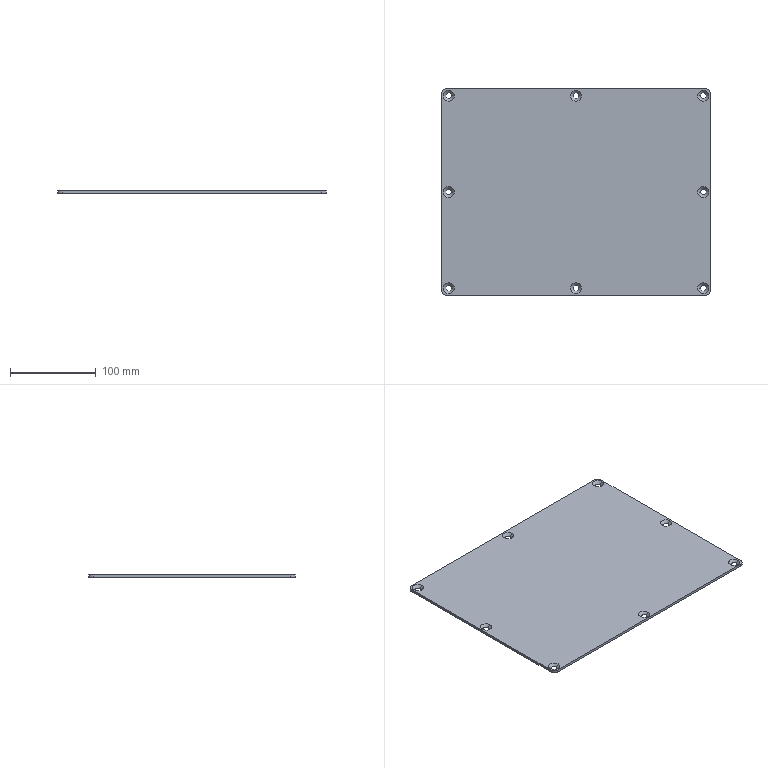Part | STEP file | PN_0001-11 Cover plate A | 1 solid | 26 faces | box 312 x 240 x 3 mm | volume 222709 mm3 | cone 16 | plane 6 | cylinder 4 | commonest cylinder face diameters 10 x4
STEP:
#1=CARTESIAN_POINT('',(-151.4,112.,0.));
#2=VERTEX_POINT('',#1);
#3=CARTESIAN_POINT('',(-144.6,112.,0.));
#4=VERTEX_POINT('',#3);
#5=CARTESIAN_POINT('',(-148.,112.,0.));
#6=DIRECTION('',(0.,0.,1.));
#7=DIRECTION('',(1.,0.,0.));
#8=AXIS2_PLACEMENT_3D('',#5,#6,#7);
#9=CIRCLE('',#8,3.4);
#10=EDGE_CURVE('',#2,#4,#9,.T.);
#11=ORIENTED_EDGE('',*,*,#10,.F.);
#12=CARTESIAN_POINT('',(-154.4,112.,3.));
#13=VERTEX_POINT('',#12);
#14=CARTESIAN_POINT('',(-154.4,112.,3.));
#15=DIRECTION('',(-0.7071,0.,0.7071));
#16=VECTOR('',#15,1000.);
#17=LINE('',#14,#16);
#18=EDGE_CURVE('',#2,#13,#17,.T.);
#19=ORIENTED_EDGE('',*,*,#18,.T.);
#20=CARTESIAN_POINT('',(-141.6,112.,3.));
#21=VERTEX_POINT('',#20);
#22=CARTESIAN_POINT('',(-148.,112.,3.));
#23=DIRECTION('',(0.,0.,1.));
#24=DIRECTION('',(1.,0.,0.));
#25=AXIS2_PLACEMENT_3D('',#22,#23,#24);
#26=CIRCLE('',#25,6.4);
#27=EDGE_CURVE('',#13,#21,#26,.T.);
#28=ORIENTED_EDGE('',*,*,#27,.T.);
#29=CARTESIAN_POINT('',(-141.6,112.,3.));
#30=DIRECTION('',(0.7071,0.,0.7071));
#31=VECTOR('',#30,1000.);
#32=LINE('',#29,#31);
#33=EDGE_CURVE('',#4,#21,#32,.T.);
#34=ORIENTED_EDGE('',*,*,#33,.F.);
#35=EDGE_LOOP('',(#11,#19,#28,#34));
#36=FACE_OUTER_BOUND('',#35,.T.);
#37=CARTESIAN_POINT('',(-148.,112.,3.));
#38=DIRECTION('',(0.,0.,1.));
#39=DIRECTION('',(1.,0.,0.));
#40=AXIS2_PLACEMENT_3D('',#37,#38,#39);
#41=CONICAL_SURFACE('',#40,6.4,0.7854);
#42=ADVANCED_FACE('',(#36),#41,.F.);
#43=CARTESIAN_POINT('',(-3.4,112.,0.));
#44=VERTEX_POINT('',#43);
#45=CARTESIAN_POINT('',(3.4,112.,0.));
#46=VERTEX_POINT('',#45);
#47=CARTESIAN_POINT('',(0.,112.,0.));
#48=DIRECTION('',(0.,0.,1.));
#49=DIRECTION('',(1.,0.,0.));
#50=AXIS2_PLACEMENT_3D('',#47,#48,#49);
#51=CIRCLE('',#50,3.4);
#52=EDGE_CURVE('',#44,#46,#51,.T.);
#53=ORIENTED_EDGE('',*,*,#52,.F.);
#54=CARTESIAN_POINT('',(-6.4,112.,3.));
#55=VERTEX_POINT('',#54);
#56=CARTESIAN_POINT('',(-6.4,112.,3.));
#57=DIRECTION('',(-0.7071,0.,0.7071));
#58=VECTOR('',#57,1000.);
#59=LINE('',#56,#58);
#60=EDGE_CURVE('',#44,#55,#59,.T.);
#61=ORIENTED_EDGE('',*,*,#60,.T.);
#62=CARTESIAN_POINT('',(6.4,112.,3.));
#63=VERTEX_POINT('',#62);
#64=CARTESIAN_POINT('',(0.,112.,3.));
#65=DIRECTION('',(0.,0.,1.));
#66=DIRECTION('',(1.,0.,0.));
#67=AXIS2_PLACEMENT_3D('',#64,#65,#66);
#68=CIRCLE('',#67,6.4);
#69=EDGE_CURVE('',#55,#63,#68,.T.);
#70=ORIENTED_EDGE('',*,*,#69,.T.);
#71=CARTESIAN_POINT('',(6.4,112.,3.));
#72=DIRECTION('',(0.7071,0.,0.7071));
#73=VECTOR('',#72,1000.);
#74=LINE('',#71,#73);
#75=EDGE_CURVE('',#46,#63,#74,.T.);
#76=ORIENTED_EDGE('',*,*,#75,.F.);
#77=EDGE_LOOP('',(#53,#61,#70,#76));
#78=FACE_OUTER_BOUND('',#77,.T.);
#79=CARTESIAN_POINT('',(0.,112.,3.));
#80=DIRECTION('',(0.,0.,1.));
#81=DIRECTION('',(1.,0.,0.));
#82=AXIS2_PLACEMENT_3D('',#79,#80,#81);
#83=CONICAL_SURFACE('',#82,6.4,0.7854);
#84=ADVANCED_FACE('',(#78),#83,.F.);
#85=CARTESIAN_POINT('',(144.6,112.,0.));
#86=VERTEX_POINT('',#85);
#87=CARTESIAN_POINT('',(151.4,112.,0.));
#88=VERTEX_POINT('',#87);
#89=CARTESIAN_POINT('',(148.,112.,0.));
#90=DIRECTION('',(0.,0.,1.));
#91=DIRECTION('',(1.,0.,0.));
#92=AXIS2_PLACEMENT_3D('',#89,#90,#91);
#93=CIRCLE('',#92,3.4);
#94=EDGE_CURVE('',#86,#88,#93,.T.);
#95=ORIENTED_EDGE('',*,*,#94,.F.);
#96=CARTESIAN_POINT('',(141.6,112.,3.));
#97=VERTEX_POINT('',#96);
#98=CARTESIAN_POINT('',(141.6,112.,3.));
#99=DIRECTION('',(-0.7071,0.,0.7071));
#100=VECTOR('',#99,1000.);
#101=LINE('',#98,#100);
#102=EDGE_CURVE('',#86,#97,#101,.T.);
#103=ORIENTED_EDGE('',*,*,#102,.T.);
#104=CARTESIAN_POINT('',(154.4,112.,3.));
#105=VERTEX_POINT('',#104);
#106=CARTESIAN_POINT('',(148.,112.,3.));
#107=DIRECTION('',(0.,0.,1.));
#108=DIRECTION('',(1.,0.,0.));
#109=AXIS2_PLACEMENT_3D('',#106,#107,#108);
#110=CIRCLE('',#109,6.4);
#111=EDGE_CURVE('',#97,#105,#110,.T.);
#112=ORIENTED_EDGE('',*,*,#111,.T.);
#113=CARTESIAN_POINT('',(154.4,112.,3.));
#114=DIRECTION('',(0.7071,0.,0.7071));
#115=VECTOR('',#114,1000.);
#116=LINE('',#113,#115);
#117=EDGE_CURVE('',#88,#105,#116,.T.);
#118=ORIENTED_EDGE('',*,*,#117,.F.);
#119=EDGE_LOOP('',(#95,#103,#112,#118));
#120=FACE_OUTER_BOUND('',#119,.T.);
#121=CARTESIAN_POINT('',(148.,112.,3.));
#122=DIRECTION('',(0.,0.,1.));
#123=DIRECTION('',(1.,0.,0.));
#124=AXIS2_PLACEMENT_3D('',#121,#122,#123);
#125=CONICAL_SURFACE('',#124,6.4,0.7854);
#126=ADVANCED_FACE('',(#120),#125,.F.);
#127=CARTESIAN_POINT('',(144.6,0.,0.));
#128=VERTEX_POINT('',#127);
#129=CARTESIAN_POINT('',(151.4,0.,0.));
#130=VERTEX_POINT('',#129);
#131=CARTESIAN_POINT('',(148.,0.,0.));
#132=DIRECTION('',(0.,0.,1.));
#133=DIRECTION('',(1.,0.,0.));
#134=AXIS2_PLACEMENT_3D('',#131,#132,#133);
#135=CIRCLE('',#134,3.4);
#136=EDGE_CURVE('',#128,#130,#135,.T.);
#137=ORIENTED_EDGE('',*,*,#136,.F.);
#138=CARTESIAN_POINT('',(141.6,0.,3.));
#139=VERTEX_POINT('',#138);
#140=CARTESIAN_POINT('',(141.6,0.,3.));
#141=DIRECTION('',(-0.7071,0.,0.7071));
#142=VECTOR('',#141,1000.);
#143=LINE('',#140,#142);
#144=EDGE_CURVE('',#128,#139,#143,.T.);
#145=ORIENTED_EDGE('',*,*,#144,.T.);
#146=CARTESIAN_POINT('',(154.4,0.,3.));
#147=VERTEX_POINT('',#146);
#148=CARTESIAN_POINT('',(148.,0.,3.));
#149=DIRECTION('',(0.,0.,1.));
#150=DIRECTION('',(1.,0.,0.));
#151=AXIS2_PLACEMENT_3D('',#148,#149,#150);
#152=CIRCLE('',#151,6.4);
#153=EDGE_CURVE('',#139,#147,#152,.T.);
#154=ORIENTED_EDGE('',*,*,#153,.T.);
#155=CARTESIAN_POINT('',(154.4,0.,3.));
#156=DIRECTION('',(0.7071,0.,0.7071));
#157=VECTOR('',#156,1000.);
#158=LINE('',#155,#157);
#159=EDGE_CURVE('',#130,#147,#158,.T.);
#160=ORIENTED_EDGE('',*,*,#159,.F.);
#161=EDGE_LOOP('',(#137,#145,#154,#160));
#162=FACE_OUTER_BOUND('',#161,.T.);
#163=CARTESIAN_POINT('',(148.,0.,3.));
#164=DIRECTION('',(0.,0.,1.));
#165=DIRECTION('',(1.,0.,0.));
#166=AXIS2_PLACEMENT_3D('',#163,#164,#165);
#167=CONICAL_SURFACE('',#166,6.4,0.7854);
#168=ADVANCED_FACE('',(#162),#167,.F.);
#169=CARTESIAN_POINT('',(144.6,-112.,0.));
#170=VERTEX_POINT('',#169);
#171=CARTESIAN_POINT('',(151.4,-112.,0.));
#172=VERTEX_POINT('',#171);
#173=CARTESIAN_POINT('',(148.,-112.,0.));
#174=DIRECTION('',(0.,0.,1.));
#175=DIRECTION('',(1.,0.,0.));
#176=AXIS2_PLACEMENT_3D('',#173,#174,#175);
#177=CIRCLE('',#176,3.4);
#178=EDGE_CURVE('',#170,#172,#177,.T.);
#179=ORIENTED_EDGE('',*,*,#178,.F.);
#180=CARTESIAN_POINT('',(141.6,-112.,3.));
#181=VERTEX_POINT('',#180);
#182=CARTESIAN_POINT('',(141.6,-112.,3.));
#183=DIRECTION('',(-0.7071,0.,0.7071));
#184=VECTOR('',#183,1000.);
#185=LINE('',#182,#184);
#186=EDGE_CURVE('',#170,#181,#185,.T.);
#187=ORIENTED_EDGE('',*,*,#186,.T.);
#188=CARTESIAN_POINT('',(154.4,-112.,3.));
#189=VERTEX_POINT('',#188);
#190=CARTESIAN_POINT('',(148.,-112.,3.));
#191=DIRECTION('',(0.,0.,1.));
#192=DIRECTION('',(1.,0.,0.));
#193=AXIS2_PLACEMENT_3D('',#190,#191,#192);
#194=CIRCLE('',#193,6.4);
#195=EDGE_CURVE('',#181,#189,#194,.T.);
#196=ORIENTED_EDGE('',*,*,#195,.T.);
#197=CARTESIAN_POINT('',(154.4,-112.,3.));
#198=DIRECTION('',(0.7071,0.,0.7071));
#199=VECTOR('',#198,1000.);
#200=LINE('',#197,#199);
#201=EDGE_CURVE('',#172,#189,#200,.T.);
#202=ORIENTED_EDGE('',*,*,#201,.F.);
#203=EDGE_LOOP('',(#179,#187,#196,#202));
#204=FACE_OUTER_BOUND('',#203,.T.);
#205=CARTESIAN_POINT('',(148.,-112.,3.));
#206=DIRECTION('',(0.,0.,1.));
#207=DIRECTION('',(1.,0.,0.));
#208=AXIS2_PLACEMENT_3D('',#205,#206,#207);
#209=CONICAL_SURFACE('',#208,6.4,0.7854);
#210=ADVANCED_FACE('',(#204),#209,.F.);
#211=CARTESIAN_POINT('',(-3.4,-112.,0.));
#212=VERTEX_POINT('',#211);
#213=CARTESIAN_POINT('',(3.4,-112.,0.));
#214=VERTEX_POINT('',#213);
#215=CARTESIAN_POINT('',(0.,-112.,0.));
#216=DIRECTION('',(0.,0.,1.));
#217=DIRECTION('',(1.,0.,0.));
#218=AXIS2_PLACEMENT_3D('',#215,#216,#217);
#219=CIRCLE('',#218,3.4);
#220=EDGE_CURVE('',#212,#214,#219,.T.);
#221=ORIENTED_EDGE('',*,*,#220,.F.);
#222=CARTESIAN_POINT('',(-6.4,-112.,3.));
#223=VERTEX_POINT('',#222);
#224=CARTESIAN_POINT('',(-6.4,-112.,3.));
#225=DIRECTION('',(-0.7071,0.,0.7071));
#226=VECTOR('',#225,1000.);
#227=LINE('',#224,#226);
#228=EDGE_CURVE('',#212,#223,#227,.T.);
#229=ORIENTED_EDGE('',*,*,#228,.T.);
#230=CARTESIAN_POINT('',(6.4,-112.,3.));
#231=VERTEX_POINT('',#230);
#232=CARTESIAN_POINT('',(0.,-112.,3.));
#233=DIRECTION('',(0.,0.,1.));
#234=DIRECTION('',(1.,0.,0.));
#235=AXIS2_PLACEMENT_3D('',#232,#233,#234);
#236=CIRCLE('',#235,6.4);
#237=EDGE_CURVE('',#223,#231,#236,.T.);
#238=ORIENTED_EDGE('',*,*,#237,.T.);
#239=CARTESIAN_POINT('',(6.4,-112.,3.));
#240=DIRECTION('',(0.7071,0.,0.7071));
#241=VECTOR('',#240,1000.);
#242=LINE('',#239,#241);
#243=EDGE_CURVE('',#214,#231,#242,.T.);
#244=ORIENTED_EDGE('',*,*,#243,.F.);
#245=EDGE_LOOP('',(#221,#229,#238,#244));
#246=FACE_OUTER_BOUND('',#245,.T.);
#247=CARTESIAN_POINT('',(0.,-112.,3.));
#248=DIRECTION('',(0.,0.,1.));
#249=DIRECTION('',(1.,0.,0.));
#250=AXIS2_PLACEMENT_3D('',#247,#248,#249);
#251=CONICAL_SURFACE('',#250,6.4,0.7854);
#252=ADVANCED_FACE('',(#246),#251,.F.);
#253=CARTESIAN_POINT('',(-151.4,-112.,0.));
#254=VERTEX_POINT('',#253);
#255=CARTESIAN_POINT('',(-144.6,-112.,0.));
#256=VERTEX_POINT('',#255);
#257=CARTESIAN_POINT('',(-148.,-112.,0.));
#258=DIRECTION('',(0.,0.,1.));
#259=DIRECTION('',(1.,0.,0.));
#260=AXIS2_PLACEMENT_3D('',#257,#258,#259);
#261=CIRCLE('',#260,3.4);
#262=EDGE_CURVE('',#254,#256,#261,.T.);
#263=ORIENTED_EDGE('',*,*,#262,.F.);
#264=CARTESIAN_POINT('',(-154.4,-112.,3.));
#265=VERTEX_POINT('',#264);
#266=CARTESIAN_POINT('',(-154.4,-112.,3.));
#267=DIRECTION('',(-0.7071,0.,0.7071));
#268=VECTOR('',#267,1000.);
#269=LINE('',#266,#268);
#270=EDGE_CURVE('',#254,#265,#269,.T.);
#271=ORIENTED_EDGE('',*,*,#270,.T.);
#272=CARTESIAN_POINT('',(-141.6,-112.,3.));
#273=VERTEX_POINT('',#272);
#274=CARTESIAN_POINT('',(-148.,-112.,3.));
#275=DIRECTION('',(0.,0.,1.));
#276=DIRECTION('',(1.,0.,0.));
#277=AXIS2_PLACEMENT_3D('',#274,#275,#276);
#278=CIRCLE('',#277,6.4);
#279=EDGE_CURVE('',#265,#273,#278,.T.);
#280=ORIENTED_EDGE('',*,*,#279,.T.);
#281=CARTESIAN_POINT('',(-141.6,-112.,3.));
#282=DIRECTION('',(0.7071,0.,0.7071));
#283=VECTOR('',#282,1000.);
#284=LINE('',#281,#283);
#285=EDGE_CURVE('',#256,#273,#284,.T.);
#286=ORIENTED_EDGE('',*,*,#285,.F.);
#287=EDGE_LOOP('',(#263,#271,#280,#286));
#288=FACE_OUTER_BOUND('',#287,.T.);
#289=CARTESIAN_POINT('',(-148.,-112.,3.));
#290=DIRECTION('',(0.,0.,1.));
#291=DIRECTION('',(1.,0.,0.));
#292=AXIS2_PLACEMENT_3D('',#289,#290,#291);
#293=CONICAL_SURFACE('',#292,6.4,0.7854);
#294=ADVANCED_FACE('',(#288),#293,.F.);
#295=CARTESIAN_POINT('',(-151.4,0.,0.));
#296=VERTEX_POINT('',#295);
#297=CARTESIAN_POINT('',(-144.6,0.,0.));
#298=VERTEX_POINT('',#297);
#299=CARTESIAN_POINT('',(-148.,0.,0.));
#300=DIRECTION('',(0.,0.,1.));
#301=DIRECTION('',(1.,0.,0.));
#302=AXIS2_PLACEMENT_3D('',#299,#300,#301);
#303=CIRCLE('',#302,3.4);
#304=EDGE_CURVE('',#296,#298,#303,.T.);
#305=ORIENTED_EDGE('',*,*,#304,.F.);
#306=CARTESIAN_POINT('',(-154.4,0.,3.));
#307=VERTEX_POINT('',#306);
#308=CARTESIAN_POINT('',(-154.4,0.,3.));
#309=DIRECTION('',(-0.7071,0.,0.7071));
#310=VECTOR('',#309,1000.);
#311=LINE('',#308,#310);
#312=EDGE_CURVE('',#296,#307,#311,.T.);
#313=ORIENTED_EDGE('',*,*,#312,.T.);
#314=CARTESIAN_POINT('',(-141.6,0.,3.));
#315=VERTEX_POINT('',#314);
#316=CARTESIAN_POINT('',(-148.,0.,3.));
#317=DIRECTION('',(0.,0.,1.));
#318=DIRECTION('',(1.,0.,0.));
#319=AXIS2_PLACEMENT_3D('',#316,#317,#318);
#320=CIRCLE('',#319,6.4);
#321=EDGE_CURVE('',#307,#315,#320,.T.);
#322=ORIENTED_EDGE('',*,*,#321,.T.);
#323=CARTESIAN_POINT('',(-141.6,0.,3.));
#324=DIRECTION('',(0.7071,0.,0.7071));
#325=VECTOR('',#324,1000.);
#326=LINE('',#323,#325);
#327=EDGE_CURVE('',#298,#315,#326,.T.);
#328=ORIENTED_EDGE('',*,*,#327,.F.);
#329=EDGE_LOOP('',(#305,#313,#322,#328));
#330=FACE_OUTER_BOUND('',#329,.T.);
#331=CARTESIAN_POINT('',(-148.,0.,3.));
#332=DIRECTION('',(0.,0.,1.));
#333=DIRECTION('',(1.,0.,0.));
#334=AXIS2_PLACEMENT_3D('',#331,#332,#333);
#335=CONICAL_SURFACE('',#334,6.4,0.7854);
#336=ADVANCED_FACE('',(#330),#335,.F.);
#337=CARTESIAN_POINT('',(-156.,115.,0.));
#338=VERTEX_POINT('',#337);
#339=CARTESIAN_POINT('',(-156.,-115.,0.));
#340=VERTEX_POINT('',#339);
#341=CARTESIAN_POINT('',(-156.,-120.,0.));
#342=DIRECTION('',(0.,-1.,0.));
#343=VECTOR('',#342,1000.);
#344=LINE('',#341,#343);
#345=EDGE_CURVE('',#338,#340,#344,.T.);
#346=ORIENTED_EDGE('',*,*,#345,.T.);
#347=CARTESIAN_POINT('',(-156.,-115.,3.));
#348=VERTEX_POINT('',#347);
#349=CARTESIAN_POINT('',(-156.,-115.,3.));
#350=DIRECTION('',(0.,0.,1.));
#351=VECTOR('',#350,1000.);
#352=LINE('',#349,#351);
#353=EDGE_CURVE('',#340,#348,#352,.T.);
#354=ORIENTED_EDGE('',*,*,#353,.T.);
#355=CARTESIAN_POINT('',(-156.,115.,3.));
#356=VERTEX_POINT('',#355);
#357=CARTESIAN_POINT('',(-156.,-120.,3.));
#358=DIRECTION('',(0.,-1.,0.));
#359=VECTOR('',#358,1000.);
#360=LINE('',#357,#359);
#361=EDGE_CURVE('',#356,#348,#360,.T.);
#362=ORIENTED_EDGE('',*,*,#361,.F.);
#363=CARTESIAN_POINT('',(-156.,115.,3.));
#364=DIRECTION('',(0.,0.,-1.));
#365=VECTOR('',#364,1000.);
#366=LINE('',#363,#365);
#367=EDGE_CURVE('',#356,#338,#366,.T.);
#368=ORIENTED_EDGE('',*,*,#367,.T.);
#369=EDGE_LOOP('',(#346,#354,#362,#368));
#370=FACE_OUTER_BOUND('',#369,.T.);
#371=CARTESIAN_POINT('',(-156.,-120.,3.));
#372=DIRECTION('',(1.,0.,0.));
#373=DIRECTION('',(0.,0.,-1.));
#374=AXIS2_PLACEMENT_3D('',#371,#372,#373);
#375=PLANE('',#374);
#376=ADVANCED_FACE('',(#370),#375,.F.);
#377=CARTESIAN_POINT('',(-151.,-120.,0.));
#378=VERTEX_POINT('',#377);
#379=CARTESIAN_POINT('',(151.,-120.,0.));
#380=VERTEX_POINT('',#379);
#381=CARTESIAN_POINT('',(156.,-120.,0.));
#382=DIRECTION('',(1.,0.,0.));
#383=VECTOR('',#382,1000.);
#384=LINE('',#381,#383);
#385=EDGE_CURVE('',#378,#380,#384,.T.);
#386=ORIENTED_EDGE('',*,*,#385,.T.);
#387=CARTESIAN_POINT('',(151.,-120.,3.));
#388=VERTEX_POINT('',#387);
#389=CARTESIAN_POINT('',(151.,-120.,3.));
#390=DIRECTION('',(0.,0.,1.));
#391=VECTOR('',#390,1000.);
#392=LINE('',#389,#391);
#393=EDGE_CURVE('',#380,#388,#392,.T.);
#394=ORIENTED_EDGE('',*,*,#393,.T.);
#395=CARTESIAN_POINT('',(-151.,-120.,3.));
#396=VERTEX_POINT('',#395);
#397=CARTESIAN_POINT('',(156.,-120.,3.));
#398=DIRECTION('',(1.,0.,0.));
#399=VECTOR('',#398,1000.);
#400=LINE('',#397,#399);
#401=EDGE_CURVE('',#396,#388,#400,.T.);
#402=ORIENTED_EDGE('',*,*,#401,.F.);
#403=CARTESIAN_POINT('',(-151.,-120.,3.));
#404=DIRECTION('',(0.,0.,-1.));
#405=VECTOR('',#404,1000.);
#406=LINE('',#403,#405);
#407=EDGE_CURVE('',#396,#378,#406,.T.);
#408=ORIENTED_EDGE('',*,*,#407,.T.);
#409=EDGE_LOOP('',(#386,#394,#402,#408));
#410=FACE_OUTER_BOUND('',#409,.T.);
#411=CARTESIAN_POINT('',(156.,-120.,3.));
#412=DIRECTION('',(0.,1.,0.));
#413=DIRECTION('',(0.,0.,1.));
#414=AXIS2_PLACEMENT_3D('',#411,#412,#413);
#415=PLANE('',#414);
#416=ADVANCED_FACE('',(#410),#415,.F.);
#417=CARTESIAN_POINT('',(156.,-115.,3.));
#418=VERTEX_POINT('',#417);
#419=CARTESIAN_POINT('',(156.,115.,3.));
#420=VERTEX_POINT('',#419);
#421=CARTESIAN_POINT('',(156.,-120.,3.));
#422=DIRECTION('',(0.,1.,0.));
#423=VECTOR('',#422,1000.);
#424=LINE('',#421,#423);
#425=EDGE_CURVE('',#418,#420,#424,.T.);
#426=ORIENTED_EDGE('',*,*,#425,.F.);
#427=CARTESIAN_POINT('',(156.,-115.,0.));
#428=VERTEX_POINT('',#427);
#429=CARTESIAN_POINT('',(156.,-115.,3.));
#430=DIRECTION('',(0.,0.,-1.));
#431=VECTOR('',#430,1000.);
#432=LINE('',#429,#431);
#433=EDGE_CURVE('',#418,#428,#432,.T.);
#434=ORIENTED_EDGE('',*,*,#433,.T.);
#435=CARTESIAN_POINT('',(156.,115.,0.));
#436=VERTEX_POINT('',#435);
#437=CARTESIAN_POINT('',(156.,-120.,0.));
#438=DIRECTION('',(0.,1.,0.));
#439=VECTOR('',#438,1000.);
#440=LINE('',#437,#439);
#441=EDGE_CURVE('',#428,#436,#440,.T.);
#442=ORIENTED_EDGE('',*,*,#441,.T.);
#443=CARTESIAN_POINT('',(156.,115.,3.));
#444=DIRECTION('',(0.,0.,1.));
#445=VECTOR('',#444,1000.);
#446=LINE('',#443,#445);
#447=EDGE_CURVE('',#436,#420,#446,.T.);
#448=ORIENTED_EDGE('',*,*,#447,.T.);
#449=EDGE_LOOP('',(#426,#434,#442,#448));
#450=FACE_OUTER_BOUND('',#449,.T.);
#451=CARTESIAN_POINT('',(156.,-120.,3.));
#452=DIRECTION('',(-1.,0.,0.));
#453=DIRECTION('',(0.,0.,1.));
#454=AXIS2_PLACEMENT_3D('',#451,#452,#453);
#455=PLANE('',#454);
#456=ADVANCED_FACE('',(#450),#455,.F.);
#457=CARTESIAN_POINT('',(151.,120.,3.));
#458=VERTEX_POINT('',#457);
#459=CARTESIAN_POINT('',(-151.,120.,3.));
#460=VERTEX_POINT('',#459);
#461=CARTESIAN_POINT('',(156.,120.,3.));
#462=DIRECTION('',(-1.,0.,0.));
#463=VECTOR('',#462,1000.);
#464=LINE('',#461,#463);
#465=EDGE_CURVE('',#458,#460,#464,.T.);
#466=ORIENTED_EDGE('',*,*,#465,.F.);
#467=CARTESIAN_POINT('',(151.,120.,0.));
#468=VERTEX_POINT('',#467);
#469=CARTESIAN_POINT('',(151.,120.,3.));
#470=DIRECTION('',(0.,0.,-1.));
#471=VECTOR('',#470,1000.);
#472=LINE('',#469,#471);
#473=EDGE_CURVE('',#458,#468,#472,.T.);
#474=ORIENTED_EDGE('',*,*,#473,.T.);
#475=CARTESIAN_POINT('',(-151.,120.,0.));
#476=VERTEX_POINT('',#475);
#477=CARTESIAN_POINT('',(156.,120.,0.));
#478=DIRECTION('',(-1.,0.,0.));
#479=VECTOR('',#478,1000.);
#480=LINE('',#477,#479);
#481=EDGE_CURVE('',#468,#476,#480,.T.);
#482=ORIENTED_EDGE('',*,*,#481,.T.);
#483=CARTESIAN_POINT('',(-151.,120.,3.));
#484=DIRECTION('',(0.,0.,1.));
#485=VECTOR('',#484,1000.);
#486=LINE('',#483,#485);
#487=EDGE_CURVE('',#476,#460,#486,.T.);
#488=ORIENTED_EDGE('',*,*,#487,.T.);
#489=EDGE_LOOP('',(#466,#474,#482,#488));
#490=FACE_OUTER_BOUND('',#489,.T.);
#491=CARTESIAN_POINT('',(156.,120.,3.));
#492=DIRECTION('',(0.,-1.,0.));
#493=DIRECTION('',(0.,0.,-1.));
#494=AXIS2_PLACEMENT_3D('',#491,#492,#493);
#495=PLANE('',#494);
#496=ADVANCED_FACE('',(#490),#495,.F.);
#497=CARTESIAN_POINT('',(-148.,112.,3.));
#498=DIRECTION('',(0.,0.,1.));
#499=DIRECTION('',(1.,0.,0.));
#500=AXIS2_PLACEMENT_3D('',#497,#498,#499);
#501=CIRCLE('',#500,6.4);
#502=EDGE_CURVE('',#21,#13,#501,.T.);
#503=ORIENTED_EDGE('',*,*,#502,.F.);
#504=ORIENTED_EDGE('',*,*,#27,.F.);
#505=EDGE_LOOP('',(#503,#504));
#506=FACE_BOUND('',#505,.T.);
#507=CARTESIAN_POINT('',(0.,112.,3.));
#508=DIRECTION('',(0.,0.,1.));
#509=DIRECTION('',(1.,0.,0.));
#510=AXIS2_PLACEMENT_3D('',#507,#508,#509);
#511=CIRCLE('',#510,6.4);
#512=EDGE_CURVE('',#63,#55,#511,.T.);
#513=ORIENTED_EDGE('',*,*,#512,.F.);
#514=ORIENTED_EDGE('',*,*,#69,.F.);
#515=EDGE_LOOP('',(#513,#514));
#516=FACE_BOUND('',#515,.T.);
#517=CARTESIAN_POINT('',(148.,112.,3.));
#518=DIRECTION('',(0.,0.,1.));
#519=DIRECTION('',(1.,0.,0.));
#520=AXIS2_PLACEMENT_3D('',#517,#518,#519);
#521=CIRCLE('',#520,6.4);
#522=EDGE_CURVE('',#105,#97,#521,.T.);
#523=ORIENTED_EDGE('',*,*,#522,.F.);
#524=ORIENTED_EDGE('',*,*,#111,.F.);
#525=EDGE_LOOP('',(#523,#524));
#526=FACE_BOUND('',#525,.T.);
#527=CARTESIAN_POINT('',(148.,0.,3.));
#528=DIRECTION('',(0.,0.,1.));
#529=DIRECTION('',(1.,0.,0.));
#530=AXIS2_PLACEMENT_3D('',#527,#528,#529);
#531=CIRCLE('',#530,6.4);
#532=EDGE_CURVE('',#147,#139,#531,.T.);
#533=ORIENTED_EDGE('',*,*,#532,.F.);
#534=ORIENTED_EDGE('',*,*,#153,.F.);
#535=EDGE_LOOP('',(#533,#534));
#536=FACE_BOUND('',#535,.T.);
#537=CARTESIAN_POINT('',(148.,-112.,3.));
#538=DIRECTION('',(0.,0.,1.));
#539=DIRECTION('',(1.,0.,0.));
#540=AXIS2_PLACEMENT_3D('',#537,#538,#539);
#541=CIRCLE('',#540,6.4);
#542=EDGE_CURVE('',#189,#181,#541,.T.);
#543=ORIENTED_EDGE('',*,*,#542,.F.);
#544=ORIENTED_EDGE('',*,*,#195,.F.);
#545=EDGE_LOOP('',(#543,#544));
#546=FACE_BOUND('',#545,.T.);
#547=CARTESIAN_POINT('',(0.,-112.,3.));
#548=DIRECTION('',(0.,0.,1.));
#549=DIRECTION('',(1.,0.,0.));
#550=AXIS2_PLACEMENT_3D('',#547,#548,#549);
#551=CIRCLE('',#550,6.4);
#552=EDGE_CURVE('',#231,#223,#551,.T.);
#553=ORIENTED_EDGE('',*,*,#552,.F.);
#554=ORIENTED_EDGE('',*,*,#237,.F.);
#555=EDGE_LOOP('',(#553,#554));
#556=FACE_BOUND('',#555,.T.);
#557=CARTESIAN_POINT('',(-148.,-112.,3.));
#558=DIRECTION('',(0.,0.,1.));
#559=DIRECTION('',(1.,0.,0.));
#560=AXIS2_PLACEMENT_3D('',#557,#558,#559);
#561=CIRCLE('',#560,6.4);
#562=EDGE_CURVE('',#273,#265,#561,.T.);
#563=ORIENTED_EDGE('',*,*,#562,.F.);
#564=ORIENTED_EDGE('',*,*,#279,.F.);
#565=EDGE_LOOP('',(#563,#564));
#566=FACE_BOUND('',#565,.T.);
#567=CARTESIAN_POINT('',(-148.,0.,3.));
#568=DIRECTION('',(0.,0.,1.));
#569=DIRECTION('',(1.,0.,0.));
#570=AXIS2_PLACEMENT_3D('',#567,#568,#569);
#571=CIRCLE('',#570,6.4);
#572=EDGE_CURVE('',#315,#307,#571,.T.);
#573=ORIENTED_EDGE('',*,*,#572,.F.);
#574=ORIENTED_EDGE('',*,*,#321,.F.);
#575=EDGE_LOOP('',(#573,#574));
#576=FACE_BOUND('',#575,.T.);
#577=ORIENTED_EDGE('',*,*,#401,.T.);
#578=CARTESIAN_POINT('',(151.,-115.,3.));
#579=DIRECTION('',(0.,0.,1.));
#580=DIRECTION('',(1.,0.,0.));
#581=AXIS2_PLACEMENT_3D('',#578,#579,#580);
#582=CIRCLE('',#581,5.);
#583=EDGE_CURVE('',#388,#418,#582,.T.);
#584=ORIENTED_EDGE('',*,*,#583,.T.);
#585=ORIENTED_EDGE('',*,*,#425,.T.);
#586=CARTESIAN_POINT('',(151.,115.,3.));
#587=DIRECTION('',(0.,0.,1.));
#588=DIRECTION('',(1.,0.,0.));
#589=AXIS2_PLACEMENT_3D('',#586,#587,#588);
#590=CIRCLE('',#589,5.);
#591=EDGE_CURVE('',#420,#458,#590,.T.);
#592=ORIENTED_EDGE('',*,*,#591,.T.);
#593=ORIENTED_EDGE('',*,*,#465,.T.);
#594=CARTESIAN_POINT('',(-151.,115.,3.));
#595=DIRECTION('',(0.,0.,1.));
#596=DIRECTION('',(1.,0.,0.));
#597=AXIS2_PLACEMENT_3D('',#594,#595,#596);
#598=CIRCLE('',#597,5.);
#599=EDGE_CURVE('',#460,#356,#598,.T.);
#600=ORIENTED_EDGE('',*,*,#599,.T.);
#601=ORIENTED_EDGE('',*,*,#361,.T.);
#602=CARTESIAN_POINT('',(-151.,-115.,3.));
#603=DIRECTION('',(0.,0.,1.));
#604=DIRECTION('',(1.,0.,0.));
#605=AXIS2_PLACEMENT_3D('',#602,#603,#604);
#606=CIRCLE('',#605,5.);
#607=EDGE_CURVE('',#348,#396,#606,.T.);
#608=ORIENTED_EDGE('',*,*,#607,.T.);
#609=EDGE_LOOP('',(#577,#584,#585,#592,#593,#600,#601,#608));
#610=FACE_OUTER_BOUND('',#609,.T.);
#611=CARTESIAN_POINT('',(0.,0.,3.));
#612=DIRECTION('',(0.,0.,1.));
#613=DIRECTION('',(1.,0.,0.));
#614=AXIS2_PLACEMENT_3D('',#611,#612,#613);
#615=PLANE('',#614);
#616=ADVANCED_FACE('',(#506,#516,#526,#536,#546,#556,#566,#576,#610),#615,.T.);
#617=CARTESIAN_POINT('',(-148.,112.,0.));
#618=DIRECTION('',(0.,0.,1.));
#619=DIRECTION('',(1.,0.,0.));
#620=AXIS2_PLACEMENT_3D('',#617,#618,#619);
#621=CIRCLE('',#620,3.4);
#622=EDGE_CURVE('',#4,#2,#621,.T.);
#623=ORIENTED_EDGE('',*,*,#622,.T.);
#624=ORIENTED_EDGE('',*,*,#10,.T.);
#625=EDGE_LOOP('',(#623,#624));
#626=FACE_BOUND('',#625,.T.);
#627=CARTESIAN_POINT('',(0.,112.,0.));
#628=DIRECTION('',(0.,0.,1.));
#629=DIRECTION('',(1.,0.,0.));
#630=AXIS2_PLACEMENT_3D('',#627,#628,#629);
#631=CIRCLE('',#630,3.4);
#632=EDGE_CURVE('',#46,#44,#631,.T.);
#633=ORIENTED_EDGE('',*,*,#632,.T.);
#634=ORIENTED_EDGE('',*,*,#52,.T.);
#635=EDGE_LOOP('',(#633,#634));
#636=FACE_BOUND('',#635,.T.);
#637=CARTESIAN_POINT('',(148.,112.,0.));
#638=DIRECTION('',(0.,0.,1.));
#639=DIRECTION('',(1.,0.,0.));
#640=AXIS2_PLACEMENT_3D('',#637,#638,#639);
#641=CIRCLE('',#640,3.4);
#642=EDGE_CURVE('',#88,#86,#641,.T.);
#643=ORIENTED_EDGE('',*,*,#642,.T.);
#644=ORIENTED_EDGE('',*,*,#94,.T.);
#645=EDGE_LOOP('',(#643,#644));
#646=FACE_BOUND('',#645,.T.);
#647=CARTESIAN_POINT('',(148.,0.,0.));
#648=DIRECTION('',(0.,0.,1.));
#649=DIRECTION('',(1.,0.,0.));
#650=AXIS2_PLACEMENT_3D('',#647,#648,#649);
#651=CIRCLE('',#650,3.4);
#652=EDGE_CURVE('',#130,#128,#651,.T.);
#653=ORIENTED_EDGE('',*,*,#652,.T.);
#654=ORIENTED_EDGE('',*,*,#136,.T.);
#655=EDGE_LOOP('',(#653,#654));
#656=FACE_BOUND('',#655,.T.);
#657=CARTESIAN_POINT('',(148.,-112.,0.));
#658=DIRECTION('',(0.,0.,1.));
#659=DIRECTION('',(1.,0.,0.));
#660=AXIS2_PLACEMENT_3D('',#657,#658,#659);
#661=CIRCLE('',#660,3.4);
#662=EDGE_CURVE('',#172,#170,#661,.T.);
#663=ORIENTED_EDGE('',*,*,#662,.T.);
#664=ORIENTED_EDGE('',*,*,#178,.T.);
#665=EDGE_LOOP('',(#663,#664));
#666=FACE_BOUND('',#665,.T.);
#667=CARTESIAN_POINT('',(0.,-112.,0.));
#668=DIRECTION('',(0.,0.,1.));
#669=DIRECTION('',(1.,0.,0.));
#670=AXIS2_PLACEMENT_3D('',#667,#668,#669);
#671=CIRCLE('',#670,3.4);
#672=EDGE_CURVE('',#214,#212,#671,.T.);
#673=ORIENTED_EDGE('',*,*,#672,.T.);
#674=ORIENTED_EDGE('',*,*,#220,.T.);
#675=EDGE_LOOP('',(#673,#674));
#676=FACE_BOUND('',#675,.T.);
#677=CARTESIAN_POINT('',(-148.,-112.,0.));
#678=DIRECTION('',(0.,0.,1.));
#679=DIRECTION('',(1.,0.,0.));
#680=AXIS2_PLACEMENT_3D('',#677,#678,#679);
#681=CIRCLE('',#680,3.4);
#682=EDGE_CURVE('',#256,#254,#681,.T.);
#683=ORIENTED_EDGE('',*,*,#682,.T.);
#684=ORIENTED_EDGE('',*,*,#262,.T.);
#685=EDGE_LOOP('',(#683,#684));
#686=FACE_BOUND('',#685,.T.);
#687=CARTESIAN_POINT('',(-148.,0.,0.));
#688=DIRECTION('',(0.,0.,1.));
#689=DIRECTION('',(1.,0.,0.));
#690=AXIS2_PLACEMENT_3D('',#687,#688,#689);
#691=CIRCLE('',#690,3.4);
#692=EDGE_CURVE('',#298,#296,#691,.T.);
#693=ORIENTED_EDGE('',*,*,#692,.T.);
#694=ORIENTED_EDGE('',*,*,#304,.T.);
#695=EDGE_LOOP('',(#693,#694));
#696=FACE_BOUND('',#695,.T.);
#697=ORIENTED_EDGE('',*,*,#441,.F.);
#698=CARTESIAN_POINT('',(151.,-115.,0.));
#699=DIRECTION('',(0.,0.,-1.));
#700=DIRECTION('',(1.,0.,0.));
#701=AXIS2_PLACEMENT_3D('',#698,#699,#700);
#702=CIRCLE('',#701,5.);
#703=EDGE_CURVE('',#428,#380,#702,.T.);
#704=ORIENTED_EDGE('',*,*,#703,.T.);
#705=ORIENTED_EDGE('',*,*,#385,.F.);
#706=CARTESIAN_POINT('',(-151.,-115.,0.));
#707=DIRECTION('',(0.,0.,-1.));
#708=DIRECTION('',(1.,0.,0.));
#709=AXIS2_PLACEMENT_3D('',#706,#707,#708);
#710=CIRCLE('',#709,5.);
#711=EDGE_CURVE('',#378,#340,#710,.T.);
#712=ORIENTED_EDGE('',*,*,#711,.T.);
#713=ORIENTED_EDGE('',*,*,#345,.F.);
#714=CARTESIAN_POINT('',(-151.,115.,0.));
#715=DIRECTION('',(0.,0.,-1.));
#716=DIRECTION('',(1.,0.,0.));
#717=AXIS2_PLACEMENT_3D('',#714,#715,#716);
#718=CIRCLE('',#717,5.);
#719=EDGE_CURVE('',#338,#476,#718,.T.);
#720=ORIENTED_EDGE('',*,*,#719,.T.);
#721=ORIENTED_EDGE('',*,*,#481,.F.);
#722=CARTESIAN_POINT('',(151.,115.,0.));
#723=DIRECTION('',(0.,0.,-1.));
#724=DIRECTION('',(1.,0.,0.));
#725=AXIS2_PLACEMENT_3D('',#722,#723,#724);
#726=CIRCLE('',#725,5.);
#727=EDGE_CURVE('',#468,#436,#726,.T.);
#728=ORIENTED_EDGE('',*,*,#727,.T.);
#729=EDGE_LOOP('',(#697,#704,#705,#712,#713,#720,#721,#728));
#730=FACE_OUTER_BOUND('',#729,.T.);
#731=CARTESIAN_POINT('',(0.,0.,0.));
#732=DIRECTION('',(0.,0.,1.));
#733=DIRECTION('',(1.,0.,0.));
#734=AXIS2_PLACEMENT_3D('',#731,#732,#733);
#735=PLANE('',#734);
#736=ADVANCED_FACE('',(#626,#636,#646,#656,#666,#676,#686,#696,#730),#735,.F.);
#737=ORIENTED_EDGE('',*,*,#583,.F.);
#738=ORIENTED_EDGE('',*,*,#393,.F.);
#739=ORIENTED_EDGE('',*,*,#703,.F.);
#740=ORIENTED_EDGE('',*,*,#433,.F.);
#741=EDGE_LOOP('',(#737,#738,#739,#740));
#742=FACE_OUTER_BOUND('',#741,.T.);
#743=CARTESIAN_POINT('',(151.,-115.,3.));
#744=DIRECTION('',(0.,0.,-1.));
#745=DIRECTION('',(-1.,0.,0.));
#746=AXIS2_PLACEMENT_3D('',#743,#744,#745);
#747=CYLINDRICAL_SURFACE('',#746,5.);
#748=ADVANCED_FACE('',(#742),#747,.T.);
#749=ORIENTED_EDGE('',*,*,#607,.F.);
#750=ORIENTED_EDGE('',*,*,#353,.F.);
#751=ORIENTED_EDGE('',*,*,#711,.F.);
#752=ORIENTED_EDGE('',*,*,#407,.F.);
#753=EDGE_LOOP('',(#749,#750,#751,#752));
#754=FACE_OUTER_BOUND('',#753,.T.);
#755=CARTESIAN_POINT('',(-151.,-115.,3.));
#756=DIRECTION('',(0.,0.,-1.));
#757=DIRECTION('',(-1.,0.,0.));
#758=AXIS2_PLACEMENT_3D('',#755,#756,#757);
#759=CYLINDRICAL_SURFACE('',#758,5.);
#760=ADVANCED_FACE('',(#754),#759,.T.);
#761=ORIENTED_EDGE('',*,*,#591,.F.);
#762=ORIENTED_EDGE('',*,*,#447,.F.);
#763=ORIENTED_EDGE('',*,*,#727,.F.);
#764=ORIENTED_EDGE('',*,*,#473,.F.);
#765=EDGE_LOOP('',(#761,#762,#763,#764));
#766=FACE_OUTER_BOUND('',#765,.T.);
#767=CARTESIAN_POINT('',(151.,115.,3.));
#768=DIRECTION('',(0.,0.,-1.));
#769=DIRECTION('',(-1.,0.,0.));
#770=AXIS2_PLACEMENT_3D('',#767,#768,#769);
#771=CYLINDRICAL_SURFACE('',#770,5.);
#772=ADVANCED_FACE('',(#766),#771,.T.);
#773=ORIENTED_EDGE('',*,*,#599,.F.);
#774=ORIENTED_EDGE('',*,*,#487,.F.);
#775=ORIENTED_EDGE('',*,*,#719,.F.);
#776=ORIENTED_EDGE('',*,*,#367,.F.);
#777=EDGE_LOOP('',(#773,#774,#775,#776));
#778=FACE_OUTER_BOUND('',#777,.T.);
#779=CARTESIAN_POINT('',(-151.,115.,3.));
#780=DIRECTION('',(0.,0.,-1.));
#781=DIRECTION('',(-1.,0.,0.));
#782=AXIS2_PLACEMENT_3D('',#779,#780,#781);
#783=CYLINDRICAL_SURFACE('',#782,5.);
#784=ADVANCED_FACE('',(#778),#783,.T.);
#785=ORIENTED_EDGE('',*,*,#312,.F.);
#786=ORIENTED_EDGE('',*,*,#692,.F.);
#787=ORIENTED_EDGE('',*,*,#327,.T.);
#788=ORIENTED_EDGE('',*,*,#572,.T.);
#789=EDGE_LOOP('',(#785,#786,#787,#788));
#790=FACE_OUTER_BOUND('',#789,.T.);
#791=CARTESIAN_POINT('',(-148.,0.,3.));
#792=DIRECTION('',(0.,0.,1.));
#793=DIRECTION('',(1.,0.,0.));
#794=AXIS2_PLACEMENT_3D('',#791,#792,#793);
#795=CONICAL_SURFACE('',#794,6.4,0.7854);
#796=ADVANCED_FACE('',(#790),#795,.F.);
#797=ORIENTED_EDGE('',*,*,#270,.F.);
#798=ORIENTED_EDGE('',*,*,#682,.F.);
#799=ORIENTED_EDGE('',*,*,#285,.T.);
#800=ORIENTED_EDGE('',*,*,#562,.T.);
#801=EDGE_LOOP('',(#797,#798,#799,#800));
#802=FACE_OUTER_BOUND('',#801,.T.);
#803=CARTESIAN_POINT('',(-148.,-112.,3.));
#804=DIRECTION('',(0.,0.,1.));
#805=DIRECTION('',(1.,0.,0.));
#806=AXIS2_PLACEMENT_3D('',#803,#804,#805);
#807=CONICAL_SURFACE('',#806,6.4,0.7854);
#808=ADVANCED_FACE('',(#802),#807,.F.);
#809=ORIENTED_EDGE('',*,*,#228,.F.);
#810=ORIENTED_EDGE('',*,*,#672,.F.);
#811=ORIENTED_EDGE('',*,*,#243,.T.);
#812=ORIENTED_EDGE('',*,*,#552,.T.);
#813=EDGE_LOOP('',(#809,#810,#811,#812));
#814=FACE_OUTER_BOUND('',#813,.T.);
#815=CARTESIAN_POINT('',(0.,-112.,3.));
#816=DIRECTION('',(0.,0.,1.));
#817=DIRECTION('',(1.,0.,0.));
#818=AXIS2_PLACEMENT_3D('',#815,#816,#817);
#819=CONICAL_SURFACE('',#818,6.4,0.7854);
#820=ADVANCED_FACE('',(#814),#819,.F.);
#821=ORIENTED_EDGE('',*,*,#186,.F.);
#822=ORIENTED_EDGE('',*,*,#662,.F.);
#823=ORIENTED_EDGE('',*,*,#201,.T.);
#824=ORIENTED_EDGE('',*,*,#542,.T.);
#825=EDGE_LOOP('',(#821,#822,#823,#824));
#826=FACE_OUTER_BOUND('',#825,.T.);
#827=CARTESIAN_POINT('',(148.,-112.,3.));
#828=DIRECTION('',(0.,0.,1.));
#829=DIRECTION('',(1.,0.,0.));
#830=AXIS2_PLACEMENT_3D('',#827,#828,#829);
#831=CONICAL_SURFACE('',#830,6.4,0.7854);
#832=ADVANCED_FACE('',(#826),#831,.F.);
#833=ORIENTED_EDGE('',*,*,#144,.F.);
#834=ORIENTED_EDGE('',*,*,#652,.F.);
#835=ORIENTED_EDGE('',*,*,#159,.T.);
#836=ORIENTED_EDGE('',*,*,#532,.T.);
#837=EDGE_LOOP('',(#833,#834,#835,#836));
#838=FACE_OUTER_BOUND('',#837,.T.);
#839=CARTESIAN_POINT('',(148.,0.,3.));
#840=DIRECTION('',(0.,0.,1.));
#841=DIRECTION('',(1.,0.,0.));
#842=AXIS2_PLACEMENT_3D('',#839,#840,#841);
#843=CONICAL_SURFACE('',#842,6.4,0.7854);
#844=ADVANCED_FACE('',(#838),#843,.F.);
#845=ORIENTED_EDGE('',*,*,#102,.F.);
#846=ORIENTED_EDGE('',*,*,#642,.F.);
#847=ORIENTED_EDGE('',*,*,#117,.T.);
#848=ORIENTED_EDGE('',*,*,#522,.T.);
#849=EDGE_LOOP('',(#845,#846,#847,#848));
#850=FACE_OUTER_BOUND('',#849,.T.);
#851=CARTESIAN_POINT('',(148.,112.,3.));
#852=DIRECTION('',(0.,0.,1.));
#853=DIRECTION('',(1.,0.,0.));
#854=AXIS2_PLACEMENT_3D('',#851,#852,#853);
#855=CONICAL_SURFACE('',#854,6.4,0.7854);
#856=ADVANCED_FACE('',(#850),#855,.F.);
#857=ORIENTED_EDGE('',*,*,#60,.F.);
#858=ORIENTED_EDGE('',*,*,#632,.F.);
#859=ORIENTED_EDGE('',*,*,#75,.T.);
#860=ORIENTED_EDGE('',*,*,#512,.T.);
#861=EDGE_LOOP('',(#857,#858,#859,#860));
#862=FACE_OUTER_BOUND('',#861,.T.);
#863=CARTESIAN_POINT('',(0.,112.,3.));
#864=DIRECTION('',(0.,0.,1.));
#865=DIRECTION('',(1.,0.,0.));
#866=AXIS2_PLACEMENT_3D('',#863,#864,#865);
#867=CONICAL_SURFACE('',#866,6.4,0.7854);
#868=ADVANCED_FACE('',(#862),#867,.F.);
#869=ORIENTED_EDGE('',*,*,#18,.F.);
#870=ORIENTED_EDGE('',*,*,#622,.F.);
#871=ORIENTED_EDGE('',*,*,#33,.T.);
#872=ORIENTED_EDGE('',*,*,#502,.T.);
#873=EDGE_LOOP('',(#869,#870,#871,#872));
#874=FACE_OUTER_BOUND('',#873,.T.);
#875=CARTESIAN_POINT('',(-148.,112.,3.));
#876=DIRECTION('',(0.,0.,1.));
#877=DIRECTION('',(1.,0.,0.));
#878=AXIS2_PLACEMENT_3D('',#875,#876,#877);
#879=CONICAL_SURFACE('',#878,6.4,0.7854);
#880=ADVANCED_FACE('',(#874),#879,.F.);
#881=CLOSED_SHELL('',(#42,#84,#126,#168,#210,#252,#294,#336,#376,#416,#456,#496,#616,#736,#748,#760,#772,#784,#796,#808,#820,#832,#844,#856,#868,#880));
#882=MANIFOLD_SOLID_BREP('',#881);
#883=CARTESIAN_POINT('',(0.,0.,0.));
#884=DIRECTION('',(0.,0.,1.));
#885=DIRECTION('',(1.,0.,0.));
#886=AXIS2_PLACEMENT_3D('',#883,#884,#885);
#887=(LENGTH_UNIT()NAMED_UNIT(*)SI_UNIT(.MILLI.,.METRE.));
#888=UNCERTAINTY_MEASURE_WITH_UNIT(LENGTH_MEASURE(0.00001),#887,'','');
#889=(NAMED_UNIT(*)PLANE_ANGLE_UNIT()SI_UNIT($,.RADIAN.));
#890=(NAMED_UNIT(*)SI_UNIT($,.STERADIAN.)SOLID_ANGLE_UNIT());
#891=(GEOMETRIC_REPRESENTATION_CONTEXT(3)GLOBAL_UNCERTAINTY_ASSIGNED_CONTEXT((#888))GLOBAL_UNIT_ASSIGNED_CONTEXT((#887,#889,#890))REPRESENTATION_CONTEXT('',''));
#892=ADVANCED_BREP_SHAPE_REPRESENTATION('',(#882,#886),#891);